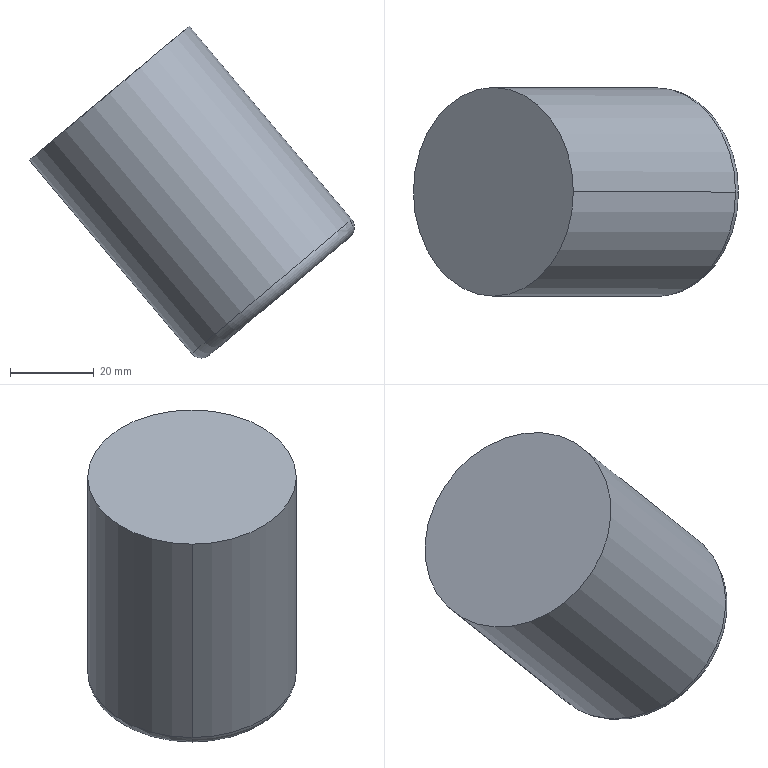Part | SolidWorks | features BaseBody 1 | 1 solid | 6 faces | box 77.861 x 50 x 79.518 mm | volume 124289 mm3 | torus 2 | cylinder 2 | plane 2 | commonest cylinder face diameters 50 x2
STEP:
#1=CARTESIAN_POINT('',(463.247,-4.,82.517));
#2=VERTEX_POINT('',#1);
#3=CARTESIAN_POINT('',(429.541,-4.,54.234));
#4=VERTEX_POINT('',#3);
#5=CARTESIAN_POINT('',(446.394,-4.,68.376));
#6=DIRECTION('',(0.6428,0.,-0.766));
#7=DIRECTION('',(0.766,0.,0.6428));
#8=AXIS2_PLACEMENT_3D('',#5,#6,#7);
#9=CIRCLE('',#8,22.);
#10=EDGE_CURVE('',#2,#4,#9,.T.);
#11=ORIENTED_EDGE('',*,*,#10,.F.);
#12=CARTESIAN_POINT('',(463.617,-4.,86.744));
#13=VERTEX_POINT('',#12);
#14=CARTESIAN_POINT('',(461.319,-4.,84.815));
#15=DIRECTION('',(0.,-1.,0.));
#16=DIRECTION('',(1.,0.,0.));
#17=AXIS2_PLACEMENT_3D('',#14,#15,#16);
#18=CIRCLE('',#17,3.);
#19=EDGE_CURVE('',#2,#13,#18,.T.);
#20=ORIENTED_EDGE('',*,*,#19,.T.);
#21=CARTESIAN_POINT('',(425.315,-4.,54.604));
#22=VERTEX_POINT('',#21);
#23=CARTESIAN_POINT('',(444.466,-4.,70.674));
#24=DIRECTION('',(-0.6428,0.,0.766));
#25=DIRECTION('',(0.766,0.,0.6428));
#26=AXIS2_PLACEMENT_3D('',#23,#24,#25);
#27=CIRCLE('',#26,25.);
#28=EDGE_CURVE('',#22,#13,#27,.T.);
#29=ORIENTED_EDGE('',*,*,#28,.F.);
#30=CARTESIAN_POINT('',(427.613,-4.,56.532));
#31=DIRECTION('',(0.,1.,0.));
#32=DIRECTION('',(0.,0.,1.));
#33=AXIS2_PLACEMENT_3D('',#30,#31,#32);
#34=CIRCLE('',#33,3.);
#35=EDGE_CURVE('',#4,#22,#34,.T.);
#36=ORIENTED_EDGE('',*,*,#35,.F.);
#37=EDGE_LOOP('',(#11,#20,#29,#36));
#38=FACE_OUTER_BOUND('',#37,.T.);
#39=CARTESIAN_POINT('',(444.466,-4.,70.674));
#40=DIRECTION('',(-0.6428,0.,0.766));
#41=DIRECTION('',(-0.766,0.,-0.6428));
#42=AXIS2_PLACEMENT_3D('',#39,#40,#41);
#43=TOROIDAL_SURFACE('',#42,22.,3.);
#44=ADVANCED_FACE('',(#38),#43,.T.);
#45=CARTESIAN_POINT('',(386.458,-4.,100.912));
#46=VERTEX_POINT('',#45);
#47=CARTESIAN_POINT('',(424.76,-4.,133.051));
#48=VERTEX_POINT('',#47);
#49=CARTESIAN_POINT('',(405.609,-4.,116.981));
#50=DIRECTION('',(-0.6428,0.,0.766));
#51=DIRECTION('',(0.766,0.,0.6428));
#52=AXIS2_PLACEMENT_3D('',#49,#50,#51);
#53=CIRCLE('',#52,25.);
#54=EDGE_CURVE('',#46,#48,#53,.T.);
#55=ORIENTED_EDGE('',*,*,#54,.F.);
#56=CARTESIAN_POINT('',(386.458,-4.,100.912));
#57=DIRECTION('',(0.6428,0.,-0.766));
#58=VECTOR('',#57,1000.);
#59=LINE('',#56,#58);
#60=EDGE_CURVE('',#46,#22,#59,.T.);
#61=ORIENTED_EDGE('',*,*,#60,.T.);
#62=ORIENTED_EDGE('',*,*,#28,.T.);
#63=CARTESIAN_POINT('',(424.76,-4.,133.051));
#64=DIRECTION('',(0.6428,0.,-0.766));
#65=VECTOR('',#64,1000.);
#66=LINE('',#63,#65);
#67=EDGE_CURVE('',#48,#13,#66,.T.);
#68=ORIENTED_EDGE('',*,*,#67,.F.);
#69=EDGE_LOOP('',(#55,#61,#62,#68));
#70=FACE_OUTER_BOUND('',#69,.T.);
#71=CARTESIAN_POINT('',(405.609,-4.,116.981));
#72=DIRECTION('',(0.6428,0.,-0.766));
#73=DIRECTION('',(0.766,0.,0.6428));
#74=AXIS2_PLACEMENT_3D('',#71,#72,#73);
#75=CYLINDRICAL_SURFACE('',#74,25.);
#76=ADVANCED_FACE('',(#70),#75,.T.);
#77=CARTESIAN_POINT('',(446.394,-4.,68.376));
#78=DIRECTION('',(0.6428,0.,-0.766));
#79=DIRECTION('',(0.766,0.,0.6428));
#80=AXIS2_PLACEMENT_3D('',#77,#78,#79);
#81=CIRCLE('',#80,22.);
#82=EDGE_CURVE('',#4,#2,#81,.T.);
#83=ORIENTED_EDGE('',*,*,#82,.T.);
#84=ORIENTED_EDGE('',*,*,#10,.T.);
#85=EDGE_LOOP('',(#83,#84));
#86=FACE_OUTER_BOUND('',#85,.T.);
#87=CARTESIAN_POINT('',(446.394,-4.,68.376));
#88=DIRECTION('',(-0.6428,0.,0.766));
#89=DIRECTION('',(0.,1.,0.));
#90=AXIS2_PLACEMENT_3D('',#87,#88,#89);
#91=PLANE('',#90);
#92=ADVANCED_FACE('',(#86),#91,.F.);
#93=CARTESIAN_POINT('',(405.609,-4.,116.981));
#94=DIRECTION('',(-0.6428,0.,0.766));
#95=DIRECTION('',(0.766,0.,0.6428));
#96=AXIS2_PLACEMENT_3D('',#93,#94,#95);
#97=CIRCLE('',#96,25.);
#98=EDGE_CURVE('',#48,#46,#97,.T.);
#99=ORIENTED_EDGE('',*,*,#98,.T.);
#100=ORIENTED_EDGE('',*,*,#54,.T.);
#101=EDGE_LOOP('',(#99,#100));
#102=FACE_OUTER_BOUND('',#101,.T.);
#103=CARTESIAN_POINT('',(405.609,-4.,116.981));
#104=DIRECTION('',(-0.6428,0.,0.766));
#105=DIRECTION('',(0.,1.,0.));
#106=AXIS2_PLACEMENT_3D('',#103,#104,#105);
#107=PLANE('',#106);
#108=ADVANCED_FACE('',(#102),#107,.T.);
#109=ORIENTED_EDGE('',*,*,#60,.F.);
#110=ORIENTED_EDGE('',*,*,#98,.F.);
#111=ORIENTED_EDGE('',*,*,#67,.T.);
#112=CARTESIAN_POINT('',(444.466,-4.,70.674));
#113=DIRECTION('',(-0.6428,0.,0.766));
#114=DIRECTION('',(0.766,0.,0.6428));
#115=AXIS2_PLACEMENT_3D('',#112,#113,#114);
#116=CIRCLE('',#115,25.);
#117=EDGE_CURVE('',#13,#22,#116,.T.);
#118=ORIENTED_EDGE('',*,*,#117,.T.);
#119=EDGE_LOOP('',(#109,#110,#111,#118));
#120=FACE_OUTER_BOUND('',#119,.T.);
#121=CARTESIAN_POINT('',(405.609,-4.,116.981));
#122=DIRECTION('',(0.6428,0.,-0.766));
#123=DIRECTION('',(0.766,0.,0.6428));
#124=AXIS2_PLACEMENT_3D('',#121,#122,#123);
#125=CYLINDRICAL_SURFACE('',#124,25.);
#126=ADVANCED_FACE('',(#120),#125,.T.);
#127=ORIENTED_EDGE('',*,*,#19,.F.);
#128=ORIENTED_EDGE('',*,*,#82,.F.);
#129=ORIENTED_EDGE('',*,*,#35,.T.);
#130=ORIENTED_EDGE('',*,*,#117,.F.);
#131=EDGE_LOOP('',(#127,#128,#129,#130));
#132=FACE_OUTER_BOUND('',#131,.T.);
#133=CARTESIAN_POINT('',(444.466,-4.,70.674));
#134=DIRECTION('',(-0.6428,0.,0.766));
#135=DIRECTION('',(-0.766,0.,-0.6428));
#136=AXIS2_PLACEMENT_3D('',#133,#134,#135);
#137=TOROIDAL_SURFACE('',#136,22.,3.);
#138=ADVANCED_FACE('',(#132),#137,.T.);
#139=CLOSED_SHELL('',(#44,#76,#92,#108,#126,#138));
#140=MANIFOLD_SOLID_BREP('',#139);
#141=CARTESIAN_POINT('',(0.,0.,0.));
#142=DIRECTION('',(0.,0.,1.));
#143=DIRECTION('',(1.,0.,0.));
#144=AXIS2_PLACEMENT_3D('',#141,#142,#143);
#145=(LENGTH_UNIT()NAMED_UNIT(*)SI_UNIT(.MILLI.,.METRE.));
#146=UNCERTAINTY_MEASURE_WITH_UNIT(LENGTH_MEASURE(0.00001),#145,'','');
#147=(NAMED_UNIT(*)PLANE_ANGLE_UNIT()SI_UNIT($,.RADIAN.));
#148=(NAMED_UNIT(*)SI_UNIT($,.STERADIAN.)SOLID_ANGLE_UNIT());
#149=(GEOMETRIC_REPRESENTATION_CONTEXT(3)GLOBAL_UNCERTAINTY_ASSIGNED_CONTEXT((#146))GLOBAL_UNIT_ASSIGNED_CONTEXT((#145,#147,#148))REPRESENTATION_CONTEXT('',''));
#150=ADVANCED_BREP_SHAPE_REPRESENTATION('',(#140,#144),#149);